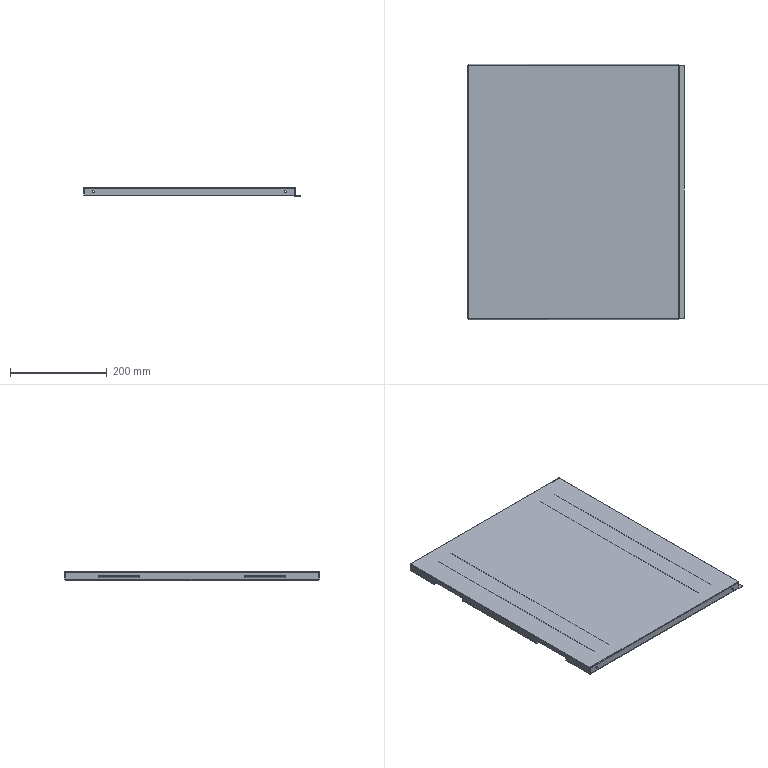Part | STEP file | 3 solids | 146 faces | box 446.8 x 526 x 18.2 mm | volume 391845 mm3 | plane 96 | cylinder 38 | spline 12 | commonest cylinder face diameters 4 x8 1 x6 3.4 x6 0.4 x4 2 x4 2.8 x4